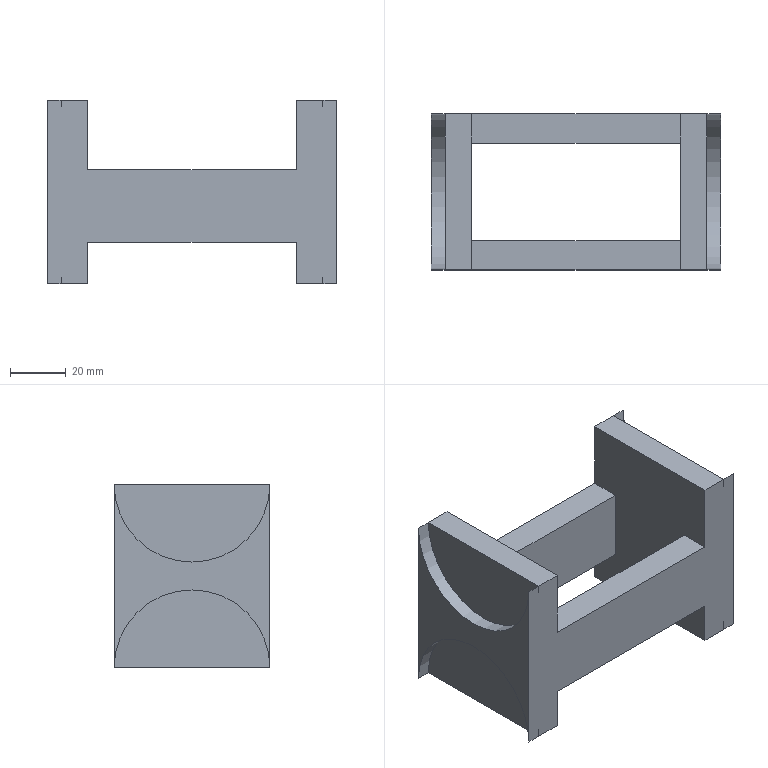Part | STEP file | Cable Carrier Part 2 | 1 solid | 24 faces | box 104 x 56 x 66 mm | volume 123504 mm3 | plane 20 | cylinder 4 | commonest cylinder face diameters 56 x4